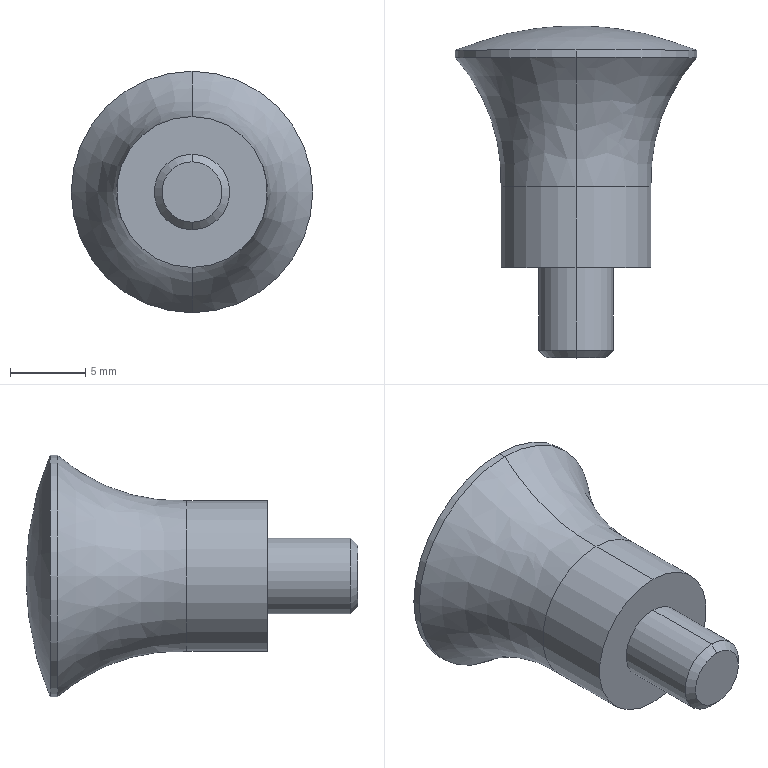Part | SolidWorks | features BaseBody 1 | 1 solid | 13 faces | box 16 x 22 x 16 mm | volume 1745 mm3 | cylinder 6 | spline 3 | cone 2 | plane 2 | commonest cylinder face diameters 5 x2 10 x2 16 x2
STEP:
#1=CARTESIAN_POINT('',(0.,11.333,-5.));
#2=VERTEX_POINT('',#1);
#3=CARTESIAN_POINT('',(0.,11.333,5.));
#4=VERTEX_POINT('',#3);
#5=CARTESIAN_POINT('',(0.,11.333,0.));
#6=DIRECTION('',(0.,-1.,0.));
#7=DIRECTION('',(0.,0.,1.));
#8=AXIS2_PLACEMENT_3D('',#5,#6,#7);
#9=CIRCLE('',#8,5.);
#10=EDGE_CURVE('',#2,#4,#9,.T.);
#11=ORIENTED_EDGE('',*,*,#10,.F.);
#12=CARTESIAN_POINT('',(0.,19.9,-8.));
#13=VERTEX_POINT('',#12);
#14=CARTESIAN_POINT('',(0.,11.945,-16.984));
#15=DIRECTION('',(-1.,0.,0.));
#16=DIRECTION('',(0.,0.,-1.));
#17=AXIS2_PLACEMENT_3D('',#14,#15,#16);
#18=CIRCLE('',#17,12.);
#19=EDGE_CURVE('',#2,#13,#18,.T.);
#20=ORIENTED_EDGE('',*,*,#19,.T.);
#21=CARTESIAN_POINT('',(0.,19.9,8.));
#22=VERTEX_POINT('',#21);
#23=CARTESIAN_POINT('',(0.,19.9,0.));
#24=DIRECTION('',(0.,1.,0.));
#25=DIRECTION('',(0.,0.,1.));
#26=AXIS2_PLACEMENT_3D('',#23,#24,#25);
#27=CIRCLE('',#26,8.);
#28=EDGE_CURVE('',#22,#13,#27,.T.);
#29=ORIENTED_EDGE('',*,*,#28,.F.);
#30=CARTESIAN_POINT('',(0.,11.945,16.984));
#31=DIRECTION('',(1.,0.,0.));
#32=DIRECTION('',(0.,0.,1.));
#33=AXIS2_PLACEMENT_3D('',#30,#31,#32);
#34=CIRCLE('',#33,12.);
#35=EDGE_CURVE('',#4,#22,#34,.T.);
#36=ORIENTED_EDGE('',*,*,#35,.F.);
#37=EDGE_LOOP('',(#11,#20,#29,#36));
#38=FACE_OUTER_BOUND('',#37,.T.);
#39=CARTESIAN_POINT('',(0.,11.333,5.));
#40=CARTESIAN_POINT('',(10.,11.333,5.));
#41=CARTESIAN_POINT('',(10.,11.333,-5.));
#42=CARTESIAN_POINT('',(0.,11.333,-5.));
#43=CARTESIAN_POINT('',(0.,14.512,4.838));
#44=CARTESIAN_POINT('',(9.675,14.512,4.838));
#45=CARTESIAN_POINT('',(9.675,14.512,-4.838));
#46=CARTESIAN_POINT('',(0.,14.512,-4.838));
#47=CARTESIAN_POINT('',(0.,17.517,5.89));
#48=CARTESIAN_POINT('',(11.78,17.517,5.89));
#49=CARTESIAN_POINT('',(11.78,17.517,-5.89));
#50=CARTESIAN_POINT('',(0.,17.517,-5.89));
#51=CARTESIAN_POINT('',(0.,19.9,8.));
#52=CARTESIAN_POINT('',(16.,19.9,8.));
#53=CARTESIAN_POINT('',(16.,19.9,-8.));
#54=CARTESIAN_POINT('',(0.,19.9,-8.));
#55=(BOUNDED_SURFACE()B_SPLINE_SURFACE(3,3,((#39,#40,#41,#42),(#43,#44,#45,#46),(#47,#48,#49,#50),(#51,#52,#53,#54)),.UNSPECIFIED.,.F.,.F.,.T.)B_SPLINE_SURFACE_WITH_KNOTS((4,4),(4,4),(0.,1.),(0.,1.),.UNSPECIFIED.)GEOMETRIC_REPRESENTATION_ITEM()RATIONAL_B_SPLINE_SURFACE(((1.,0.3333,0.3333,1.),(0.9505,0.3168,0.3168,0.9505),(0.9505,0.3168,0.3168,0.9505),(1.,0.3333,0.3333,1.)))REPRESENTATION_ITEM('')SURFACE());
#56=ADVANCED_FACE('',(#38),#55,.F.);
#57=ORIENTED_EDGE('',*,*,#10,.T.);
#58=CARTESIAN_POINT('',(0.,6.,5.));
#59=VERTEX_POINT('',#58);
#60=CARTESIAN_POINT('',(0.,50.,5.));
#61=DIRECTION('',(0.,-1.,0.));
#62=VECTOR('',#61,1000.);
#63=LINE('',#60,#62);
#64=EDGE_CURVE('',#4,#59,#63,.T.);
#65=ORIENTED_EDGE('',*,*,#64,.T.);
#66=CARTESIAN_POINT('',(0.,6.,-5.));
#67=VERTEX_POINT('',#66);
#68=CARTESIAN_POINT('',(0.,6.,0.));
#69=DIRECTION('',(0.,1.,0.));
#70=DIRECTION('',(0.,0.,-1.));
#71=AXIS2_PLACEMENT_3D('',#68,#69,#70);
#72=CIRCLE('',#71,5.);
#73=EDGE_CURVE('',#59,#67,#72,.T.);
#74=ORIENTED_EDGE('',*,*,#73,.T.);
#75=CARTESIAN_POINT('',(0.,50.,-5.));
#76=DIRECTION('',(0.,-1.,0.));
#77=VECTOR('',#76,1000.);
#78=LINE('',#75,#77);
#79=EDGE_CURVE('',#2,#67,#78,.T.);
#80=ORIENTED_EDGE('',*,*,#79,.F.);
#81=EDGE_LOOP('',(#57,#65,#74,#80));
#82=FACE_OUTER_BOUND('',#81,.T.);
#83=CARTESIAN_POINT('',(0.,50.,0.));
#84=DIRECTION('',(0.,-1.,0.));
#85=DIRECTION('',(0.,0.,-1.));
#86=AXIS2_PLACEMENT_3D('',#83,#84,#85);
#87=CYLINDRICAL_SURFACE('',#86,5.);
#88=ADVANCED_FACE('',(#82),#87,.T.);
#89=CARTESIAN_POINT('',(0.,20.4,-8.));
#90=VERTEX_POINT('',#89);
#91=CARTESIAN_POINT('',(0.,20.4,8.));
#92=VERTEX_POINT('',#91);
#93=CARTESIAN_POINT('',(0.,20.4,0.));
#94=DIRECTION('',(0.,-1.,0.));
#95=DIRECTION('',(0.,0.,-1.));
#96=AXIS2_PLACEMENT_3D('',#93,#94,#95);
#97=CIRCLE('',#96,8.);
#98=EDGE_CURVE('',#90,#92,#97,.T.);
#99=ORIENTED_EDGE('',*,*,#98,.T.);
#100=CARTESIAN_POINT('',(0.,50.,8.));
#101=DIRECTION('',(0.,-1.,0.));
#102=VECTOR('',#101,1000.);
#103=LINE('',#100,#102);
#104=EDGE_CURVE('',#92,#22,#103,.T.);
#105=ORIENTED_EDGE('',*,*,#104,.T.);
#106=ORIENTED_EDGE('',*,*,#28,.T.);
#107=CARTESIAN_POINT('',(0.,50.,-8.));
#108=DIRECTION('',(0.,-1.,0.));
#109=VECTOR('',#108,1000.);
#110=LINE('',#107,#109);
#111=EDGE_CURVE('',#90,#13,#110,.T.);
#112=ORIENTED_EDGE('',*,*,#111,.F.);
#113=EDGE_LOOP('',(#99,#105,#106,#112));
#114=FACE_OUTER_BOUND('',#113,.T.);
#115=CARTESIAN_POINT('',(0.,50.,0.));
#116=DIRECTION('',(0.,-1.,0.));
#117=DIRECTION('',(0.,0.,-1.));
#118=AXIS2_PLACEMENT_3D('',#115,#116,#117);
#119=CYLINDRICAL_SURFACE('',#118,8.);
#120=ADVANCED_FACE('',(#114),#119,.T.);
#121=CARTESIAN_POINT('',(0.,6.,-2.5));
#122=VERTEX_POINT('',#121);
#123=CARTESIAN_POINT('',(0.,6.,2.5));
#124=VERTEX_POINT('',#123);
#125=CARTESIAN_POINT('',(0.,6.,0.));
#126=DIRECTION('',(0.,-1.,0.));
#127=DIRECTION('',(0.,0.,-1.));
#128=AXIS2_PLACEMENT_3D('',#125,#126,#127);
#129=CIRCLE('',#128,2.5);
#130=EDGE_CURVE('',#122,#124,#129,.T.);
#131=ORIENTED_EDGE('',*,*,#130,.T.);
#132=CARTESIAN_POINT('',(0.,0.5,2.5));
#133=VERTEX_POINT('',#132);
#134=CARTESIAN_POINT('',(0.,50.,2.5));
#135=DIRECTION('',(0.,-1.,0.));
#136=VECTOR('',#135,1000.);
#137=LINE('',#134,#136);
#138=EDGE_CURVE('',#124,#133,#137,.T.);
#139=ORIENTED_EDGE('',*,*,#138,.T.);
#140=CARTESIAN_POINT('',(0.,0.5,-2.5));
#141=VERTEX_POINT('',#140);
#142=CARTESIAN_POINT('',(0.,0.5,0.));
#143=DIRECTION('',(0.,1.,0.));
#144=DIRECTION('',(0.,0.,-1.));
#145=AXIS2_PLACEMENT_3D('',#142,#143,#144);
#146=CIRCLE('',#145,2.5);
#147=EDGE_CURVE('',#133,#141,#146,.T.);
#148=ORIENTED_EDGE('',*,*,#147,.T.);
#149=CARTESIAN_POINT('',(0.,50.,-2.5));
#150=DIRECTION('',(0.,-1.,0.));
#151=VECTOR('',#150,1000.);
#152=LINE('',#149,#151);
#153=EDGE_CURVE('',#122,#141,#152,.T.);
#154=ORIENTED_EDGE('',*,*,#153,.F.);
#155=EDGE_LOOP('',(#131,#139,#148,#154));
#156=FACE_OUTER_BOUND('',#155,.T.);
#157=CARTESIAN_POINT('',(0.,50.,0.));
#158=DIRECTION('',(0.,-1.,0.));
#159=DIRECTION('',(0.,0.,-1.));
#160=AXIS2_PLACEMENT_3D('',#157,#158,#159);
#161=CYLINDRICAL_SURFACE('',#160,2.5);
#162=ADVANCED_FACE('',(#156),#161,.T.);
#163=CARTESIAN_POINT('',(0.,0.,2.));
#164=VERTEX_POINT('',#163);
#165=CARTESIAN_POINT('',(0.,0.,-2.));
#166=VERTEX_POINT('',#165);
#167=CARTESIAN_POINT('',(0.,0.,0.));
#168=DIRECTION('',(0.,1.,0.));
#169=DIRECTION('',(0.,0.,1.));
#170=AXIS2_PLACEMENT_3D('',#167,#168,#169);
#171=CIRCLE('',#170,2.);
#172=EDGE_CURVE('',#164,#166,#171,.T.);
#173=ORIENTED_EDGE('',*,*,#172,.T.);
#174=CARTESIAN_POINT('',(0.,0.5,-2.5));
#175=DIRECTION('',(0.,0.7071,-0.7071));
#176=VECTOR('',#175,1000.);
#177=LINE('',#174,#176);
#178=EDGE_CURVE('',#166,#141,#177,.T.);
#179=ORIENTED_EDGE('',*,*,#178,.T.);
#180=ORIENTED_EDGE('',*,*,#147,.F.);
#181=CARTESIAN_POINT('',(0.,0.5,2.5));
#182=DIRECTION('',(0.,0.7071,0.7071));
#183=VECTOR('',#182,1000.);
#184=LINE('',#181,#183);
#185=EDGE_CURVE('',#164,#133,#184,.T.);
#186=ORIENTED_EDGE('',*,*,#185,.F.);
#187=EDGE_LOOP('',(#173,#179,#180,#186));
#188=FACE_OUTER_BOUND('',#187,.T.);
#189=CARTESIAN_POINT('',(0.,0.5,0.));
#190=DIRECTION('',(0.,1.,0.));
#191=DIRECTION('',(0.,0.,1.));
#192=AXIS2_PLACEMENT_3D('',#189,#190,#191);
#193=CONICAL_SURFACE('',#192,2.5,0.7854);
#194=ADVANCED_FACE('',(#188),#193,.T.);
#195=ORIENTED_EDGE('',*,*,#19,.F.);
#196=CARTESIAN_POINT('',(0.,11.333,0.));
#197=DIRECTION('',(0.,-1.,0.));
#198=DIRECTION('',(0.,0.,1.));
#199=AXIS2_PLACEMENT_3D('',#196,#197,#198);
#200=CIRCLE('',#199,5.);
#201=EDGE_CURVE('',#4,#2,#200,.T.);
#202=ORIENTED_EDGE('',*,*,#201,.F.);
#203=ORIENTED_EDGE('',*,*,#35,.T.);
#204=CARTESIAN_POINT('',(0.,19.9,0.));
#205=DIRECTION('',(0.,1.,0.));
#206=DIRECTION('',(0.,0.,1.));
#207=AXIS2_PLACEMENT_3D('',#204,#205,#206);
#208=CIRCLE('',#207,8.);
#209=EDGE_CURVE('',#13,#22,#208,.T.);
#210=ORIENTED_EDGE('',*,*,#209,.F.);
#211=EDGE_LOOP('',(#195,#202,#203,#210));
#212=FACE_OUTER_BOUND('',#211,.T.);
#213=CARTESIAN_POINT('',(0.,11.333,-5.));
#214=CARTESIAN_POINT('',(-10.,11.333,-5.));
#215=CARTESIAN_POINT('',(-10.,11.333,5.));
#216=CARTESIAN_POINT('',(0.,11.333,5.));
#217=CARTESIAN_POINT('',(0.,14.512,-4.838));
#218=CARTESIAN_POINT('',(-9.675,14.512,-4.838));
#219=CARTESIAN_POINT('',(-9.675,14.512,4.838));
#220=CARTESIAN_POINT('',(0.,14.512,4.838));
#221=CARTESIAN_POINT('',(0.,17.517,-5.89));
#222=CARTESIAN_POINT('',(-11.78,17.517,-5.89));
#223=CARTESIAN_POINT('',(-11.78,17.517,5.89));
#224=CARTESIAN_POINT('',(0.,17.517,5.89));
#225=CARTESIAN_POINT('',(0.,19.9,-8.));
#226=CARTESIAN_POINT('',(-16.,19.9,-8.));
#227=CARTESIAN_POINT('',(-16.,19.9,8.));
#228=CARTESIAN_POINT('',(0.,19.9,8.));
#229=(BOUNDED_SURFACE()B_SPLINE_SURFACE(3,3,((#213,#214,#215,#216),(#217,#218,#219,#220),(#221,#222,#223,#224),(#225,#226,#227,#228)),.UNSPECIFIED.,.F.,.F.,.F.)B_SPLINE_SURFACE_WITH_KNOTS((4,4),(4,4),(0.,1.),(0.,1.),.UNSPECIFIED.)GEOMETRIC_REPRESENTATION_ITEM()RATIONAL_B_SPLINE_SURFACE(((1.,0.3333,0.3333,1.),(0.9505,0.3168,0.3168,0.9505),(0.9505,0.3168,0.3168,0.9505),(1.,0.3333,0.3333,1.)))REPRESENTATION_ITEM('')SURFACE());
#230=ADVANCED_FACE('',(#212),#229,.F.);
#231=ORIENTED_EDGE('',*,*,#64,.F.);
#232=ORIENTED_EDGE('',*,*,#201,.T.);
#233=ORIENTED_EDGE('',*,*,#79,.T.);
#234=CARTESIAN_POINT('',(0.,6.,0.));
#235=DIRECTION('',(0.,1.,0.));
#236=DIRECTION('',(0.,0.,-1.));
#237=AXIS2_PLACEMENT_3D('',#234,#235,#236);
#238=CIRCLE('',#237,5.);
#239=EDGE_CURVE('',#67,#59,#238,.T.);
#240=ORIENTED_EDGE('',*,*,#239,.T.);
#241=EDGE_LOOP('',(#231,#232,#233,#240));
#242=FACE_OUTER_BOUND('',#241,.T.);
#243=CARTESIAN_POINT('',(0.,50.,0.));
#244=DIRECTION('',(0.,-1.,0.));
#245=DIRECTION('',(0.,0.,-1.));
#246=AXIS2_PLACEMENT_3D('',#243,#244,#245);
#247=CYLINDRICAL_SURFACE('',#246,5.);
#248=ADVANCED_FACE('',(#242),#247,.T.);
#249=ORIENTED_EDGE('',*,*,#104,.F.);
#250=CARTESIAN_POINT('',(0.,20.4,0.));
#251=DIRECTION('',(0.,-1.,0.));
#252=DIRECTION('',(0.,0.,-1.));
#253=AXIS2_PLACEMENT_3D('',#250,#251,#252);
#254=CIRCLE('',#253,8.);
#255=EDGE_CURVE('',#92,#90,#254,.T.);
#256=ORIENTED_EDGE('',*,*,#255,.T.);
#257=ORIENTED_EDGE('',*,*,#111,.T.);
#258=ORIENTED_EDGE('',*,*,#209,.T.);
#259=EDGE_LOOP('',(#249,#256,#257,#258));
#260=FACE_OUTER_BOUND('',#259,.T.);
#261=CARTESIAN_POINT('',(0.,50.,0.));
#262=DIRECTION('',(0.,-1.,0.));
#263=DIRECTION('',(0.,0.,-1.));
#264=AXIS2_PLACEMENT_3D('',#261,#262,#263);
#265=CYLINDRICAL_SURFACE('',#264,8.);
#266=ADVANCED_FACE('',(#260),#265,.T.);
#267=ORIENTED_EDGE('',*,*,#130,.F.);
#268=CARTESIAN_POINT('',(0.,6.,0.));
#269=DIRECTION('',(0.,-1.,0.));
#270=DIRECTION('',(0.,0.,-1.));
#271=AXIS2_PLACEMENT_3D('',#268,#269,#270);
#272=CIRCLE('',#271,2.5);
#273=EDGE_CURVE('',#124,#122,#272,.T.);
#274=ORIENTED_EDGE('',*,*,#273,.F.);
#275=EDGE_LOOP('',(#267,#274));
#276=FACE_BOUND('',#275,.T.);
#277=ORIENTED_EDGE('',*,*,#239,.F.);
#278=ORIENTED_EDGE('',*,*,#73,.F.);
#279=EDGE_LOOP('',(#277,#278));
#280=FACE_OUTER_BOUND('',#279,.T.);
#281=CARTESIAN_POINT('',(0.,6.,2.5));
#282=DIRECTION('',(0.,1.,0.));
#283=DIRECTION('',(0.,0.,1.));
#284=AXIS2_PLACEMENT_3D('',#281,#282,#283);
#285=PLANE('',#284);
#286=ADVANCED_FACE('',(#276,#280),#285,.F.);
#287=ORIENTED_EDGE('',*,*,#98,.F.);
#288=ORIENTED_EDGE('',*,*,#255,.F.);
#289=EDGE_LOOP('',(#287,#288));
#290=FACE_OUTER_BOUND('',#289,.T.);
#291=CARTESIAN_POINT('',(-7.468,18.825,-8.139));
#292=CARTESIAN_POINT('',(-2.618,20.879,-8.139));
#293=CARTESIAN_POINT('',(2.648,20.875,-8.139));
#294=CARTESIAN_POINT('',(7.495,18.813,-8.139));
#295=CARTESIAN_POINT('',(-8.34,20.883,-2.883));
#296=CARTESIAN_POINT('',(-2.924,23.177,-2.883));
#297=CARTESIAN_POINT('',(2.958,23.173,-2.883));
#298=CARTESIAN_POINT('',(8.37,20.87,-2.883));
#299=CARTESIAN_POINT('',(-8.342,20.889,2.829));
#300=CARTESIAN_POINT('',(-2.925,23.185,2.829));
#301=CARTESIAN_POINT('',(2.959,23.18,2.829));
#302=CARTESIAN_POINT('',(8.373,20.876,2.829));
#303=CARTESIAN_POINT('',(-7.476,18.843,8.091));
#304=CARTESIAN_POINT('',(-2.621,20.9,8.091));
#305=CARTESIAN_POINT('',(2.651,20.896,8.091));
#306=CARTESIAN_POINT('',(7.503,18.832,8.091));
#307=(BOUNDED_SURFACE()B_SPLINE_SURFACE(3,3,((#291,#292,#293,#294),(#295,#296,#297,#298),(#299,#300,#301,#302),(#303,#304,#305,#306)),.UNSPECIFIED.,.F.,.F.,.T.)B_SPLINE_SURFACE_WITH_KNOTS((4,4),(4,4),(0.,1.),(0.,1.),.UNSPECIFIED.)GEOMETRIC_REPRESENTATION_ITEM()RATIONAL_B_SPLINE_SURFACE(((1.,0.947,0.947,1.),(0.9472,0.8969,0.8969,0.9472),(0.9472,0.8969,0.8969,0.9472),(1.,0.947,0.947,1.)))REPRESENTATION_ITEM('')SURFACE());
#308=ADVANCED_FACE('',(#290),#307,.T.);
#309=ORIENTED_EDGE('',*,*,#138,.F.);
#310=ORIENTED_EDGE('',*,*,#273,.T.);
#311=ORIENTED_EDGE('',*,*,#153,.T.);
#312=CARTESIAN_POINT('',(0.,0.5,0.));
#313=DIRECTION('',(0.,1.,0.));
#314=DIRECTION('',(0.,0.,-1.));
#315=AXIS2_PLACEMENT_3D('',#312,#313,#314);
#316=CIRCLE('',#315,2.5);
#317=EDGE_CURVE('',#141,#133,#316,.T.);
#318=ORIENTED_EDGE('',*,*,#317,.T.);
#319=EDGE_LOOP('',(#309,#310,#311,#318));
#320=FACE_OUTER_BOUND('',#319,.T.);
#321=CARTESIAN_POINT('',(0.,50.,0.));
#322=DIRECTION('',(0.,-1.,0.));
#323=DIRECTION('',(0.,0.,-1.));
#324=AXIS2_PLACEMENT_3D('',#321,#322,#323);
#325=CYLINDRICAL_SURFACE('',#324,2.5);
#326=ADVANCED_FACE('',(#320),#325,.T.);
#327=ORIENTED_EDGE('',*,*,#178,.F.);
#328=CARTESIAN_POINT('',(0.,0.,0.));
#329=DIRECTION('',(0.,1.,0.));
#330=DIRECTION('',(0.,0.,1.));
#331=AXIS2_PLACEMENT_3D('',#328,#329,#330);
#332=CIRCLE('',#331,2.);
#333=EDGE_CURVE('',#166,#164,#332,.T.);
#334=ORIENTED_EDGE('',*,*,#333,.T.);
#335=ORIENTED_EDGE('',*,*,#185,.T.);
#336=ORIENTED_EDGE('',*,*,#317,.F.);
#337=EDGE_LOOP('',(#327,#334,#335,#336));
#338=FACE_OUTER_BOUND('',#337,.T.);
#339=CARTESIAN_POINT('',(0.,0.5,0.));
#340=DIRECTION('',(0.,1.,0.));
#341=DIRECTION('',(0.,0.,1.));
#342=AXIS2_PLACEMENT_3D('',#339,#340,#341);
#343=CONICAL_SURFACE('',#342,2.5,0.7854);
#344=ADVANCED_FACE('',(#338),#343,.T.);
#345=ORIENTED_EDGE('',*,*,#172,.F.);
#346=ORIENTED_EDGE('',*,*,#333,.F.);
#347=EDGE_LOOP('',(#345,#346));
#348=FACE_OUTER_BOUND('',#347,.T.);
#349=CARTESIAN_POINT('',(0.,0.,0.));
#350=DIRECTION('',(0.,1.,0.));
#351=DIRECTION('',(0.,0.,1.));
#352=AXIS2_PLACEMENT_3D('',#349,#350,#351);
#353=PLANE('',#352);
#354=ADVANCED_FACE('',(#348),#353,.F.);
#355=CLOSED_SHELL('',(#56,#88,#120,#162,#194,#230,#248,#266,#286,#308,#326,#344,#354));
#356=MANIFOLD_SOLID_BREP('',#355);
#357=CARTESIAN_POINT('',(0.,0.,0.));
#358=DIRECTION('',(0.,0.,1.));
#359=DIRECTION('',(1.,0.,0.));
#360=AXIS2_PLACEMENT_3D('',#357,#358,#359);
#361=(LENGTH_UNIT()NAMED_UNIT(*)SI_UNIT(.MILLI.,.METRE.));
#362=UNCERTAINTY_MEASURE_WITH_UNIT(LENGTH_MEASURE(0.00001),#361,'','');
#363=(NAMED_UNIT(*)PLANE_ANGLE_UNIT()SI_UNIT($,.RADIAN.));
#364=(NAMED_UNIT(*)SI_UNIT($,.STERADIAN.)SOLID_ANGLE_UNIT());
#365=(GEOMETRIC_REPRESENTATION_CONTEXT(3)GLOBAL_UNCERTAINTY_ASSIGNED_CONTEXT((#362))GLOBAL_UNIT_ASSIGNED_CONTEXT((#361,#363,#364))REPRESENTATION_CONTEXT('',''));
#366=ADVANCED_BREP_SHAPE_REPRESENTATION('',(#356,#360),#365);